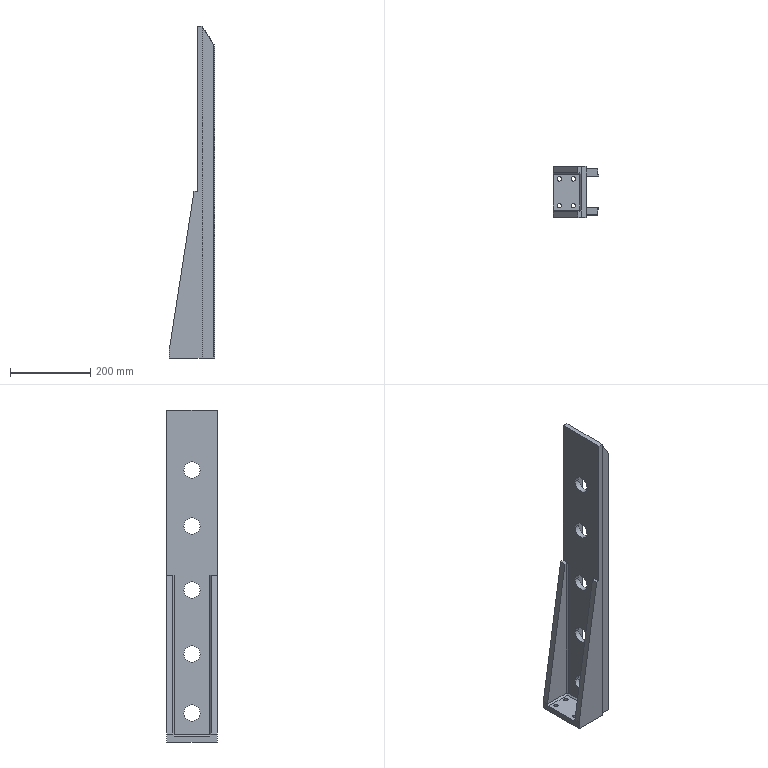Part | Creo | features CURVE 5, PROTRUSION 4, DATUM PLANE 3, CUT 2, CHAMFER 1, COORDINATE SYSTEM 1, MIRROR 1 | 1 solid | 51 faces | box 113.505 x 127.005 x 830 mm | volume 2691815 mm3 | plane 33 | cylinder 18 | commonest cylinder face diameters 40.92 x10 11 x8